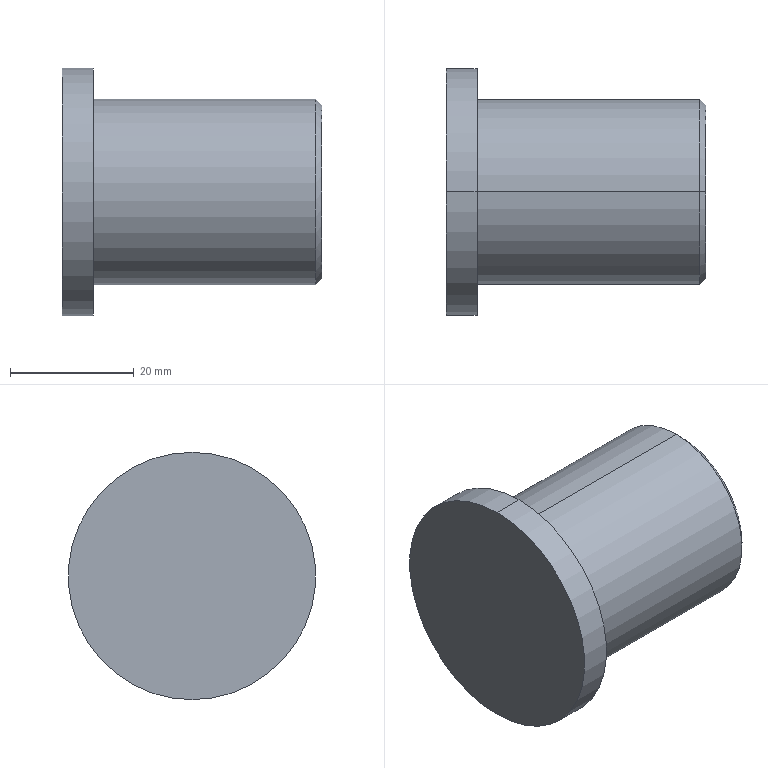Part | SolidWorks | features MBimport 1 | 1 solid | 18 faces | box 42 x 40 x 40 mm | volume 30182 mm3 | cylinder 8 | cone 6 | plane 4 | commonest cylinder face diameters 10.2 x2 12 x2 30 x2 40 x2
STEP:
#1=CARTESIAN_POINT('',(42.,17.24,-25.419));
#2=VERTEX_POINT('',#1);
#3=CARTESIAN_POINT('',(41.,17.24,-26.419));
#4=VERTEX_POINT('',#3);
#5=CARTESIAN_POINT('',(42.,17.24,-25.419));
#6=DIRECTION('',(-0.7071,0.,-0.7071));
#7=VECTOR('',#6,1000.);
#8=LINE('',#5,#7);
#9=EDGE_CURVE('',#2,#4,#8,.T.);
#10=ORIENTED_EDGE('',*,*,#9,.F.);
#11=CARTESIAN_POINT('',(42.,17.24,2.581));
#12=VERTEX_POINT('',#11);
#13=CARTESIAN_POINT('',(42.,17.24,-11.419));
#14=DIRECTION('',(1.,0.,0.));
#15=DIRECTION('',(0.,0.,-1.));
#16=AXIS2_PLACEMENT_3D('',#13,#14,#15);
#17=CIRCLE('',#16,14.);
#18=EDGE_CURVE('',#12,#2,#17,.T.);
#19=ORIENTED_EDGE('',*,*,#18,.F.);
#20=CARTESIAN_POINT('',(41.,17.24,3.581));
#21=VERTEX_POINT('',#20);
#22=CARTESIAN_POINT('',(42.,17.24,2.581));
#23=DIRECTION('',(-0.7071,0.,0.7071));
#24=VECTOR('',#23,1000.);
#25=LINE('',#22,#24);
#26=EDGE_CURVE('',#12,#21,#25,.T.);
#27=ORIENTED_EDGE('',*,*,#26,.T.);
#28=CARTESIAN_POINT('',(41.,17.24,-11.419));
#29=DIRECTION('',(-1.,0.,0.));
#30=DIRECTION('',(0.,0.,-1.));
#31=AXIS2_PLACEMENT_3D('',#28,#29,#30);
#32=CIRCLE('',#31,15.);
#33=EDGE_CURVE('',#4,#21,#32,.T.);
#34=ORIENTED_EDGE('',*,*,#33,.F.);
#35=EDGE_LOOP('',(#10,#19,#27,#34));
#36=FACE_OUTER_BOUND('',#35,.T.);
#37=CARTESIAN_POINT('',(42.,17.24,-11.419));
#38=DIRECTION('',(-1.,0.,0.));
#39=DIRECTION('',(0.,0.,1.));
#40=AXIS2_PLACEMENT_3D('',#37,#38,#39);
#41=CONICAL_SURFACE('',#40,14.,0.7854);
#42=ADVANCED_FACE('',(#36),#41,.T.);
#43=CARTESIAN_POINT('',(41.975,17.24,-5.419));
#44=VERTEX_POINT('',#43);
#45=CARTESIAN_POINT('',(42.,17.24,-5.394));
#46=VERTEX_POINT('',#45);
#47=CARTESIAN_POINT('',(42.,17.24,-5.394));
#48=DIRECTION('',(0.7071,0.,0.7071));
#49=VECTOR('',#48,1000.);
#50=LINE('',#47,#49);
#51=EDGE_CURVE('',#44,#46,#50,.T.);
#52=ORIENTED_EDGE('',*,*,#51,.F.);
#53=CARTESIAN_POINT('',(41.975,17.24,-17.419));
#54=VERTEX_POINT('',#53);
#55=CARTESIAN_POINT('',(41.975,17.24,-11.419));
#56=DIRECTION('',(1.,0.,0.));
#57=DIRECTION('',(0.,0.,-1.));
#58=AXIS2_PLACEMENT_3D('',#55,#56,#57);
#59=CIRCLE('',#58,6.);
#60=EDGE_CURVE('',#54,#44,#59,.T.);
#61=ORIENTED_EDGE('',*,*,#60,.F.);
#62=CARTESIAN_POINT('',(42.,17.24,-17.444));
#63=VERTEX_POINT('',#62);
#64=CARTESIAN_POINT('',(42.,17.24,-17.444));
#65=DIRECTION('',(0.7071,0.,-0.7071));
#66=VECTOR('',#65,1000.);
#67=LINE('',#64,#66);
#68=EDGE_CURVE('',#54,#63,#67,.T.);
#69=ORIENTED_EDGE('',*,*,#68,.T.);
#70=CARTESIAN_POINT('',(42.,17.24,-11.419));
#71=DIRECTION('',(1.,0.,0.));
#72=DIRECTION('',(0.,0.,-1.));
#73=AXIS2_PLACEMENT_3D('',#70,#71,#72);
#74=CIRCLE('',#73,6.025);
#75=EDGE_CURVE('',#63,#46,#74,.T.);
#76=ORIENTED_EDGE('',*,*,#75,.T.);
#77=EDGE_LOOP('',(#52,#61,#69,#76));
#78=FACE_OUTER_BOUND('',#77,.T.);
#79=CARTESIAN_POINT('',(42.,17.24,-11.419));
#80=DIRECTION('',(1.,0.,0.));
#81=DIRECTION('',(0.,0.,-1.));
#82=AXIS2_PLACEMENT_3D('',#79,#80,#81);
#83=CONICAL_SURFACE('',#82,6.025,0.7854);
#84=ADVANCED_FACE('',(#78),#83,.F.);
#85=CARTESIAN_POINT('',(27.,17.24,-5.419));
#86=VERTEX_POINT('',#85);
#87=CARTESIAN_POINT('',(42.,17.24,-5.419));
#88=DIRECTION('',(1.,0.,0.));
#89=VECTOR('',#88,1000.);
#90=LINE('',#87,#89);
#91=EDGE_CURVE('',#86,#44,#90,.T.);
#92=ORIENTED_EDGE('',*,*,#91,.F.);
#93=CARTESIAN_POINT('',(27.,17.24,-17.419));
#94=VERTEX_POINT('',#93);
#95=CARTESIAN_POINT('',(27.,17.24,-11.419));
#96=DIRECTION('',(1.,0.,0.));
#97=DIRECTION('',(0.,0.,-1.));
#98=AXIS2_PLACEMENT_3D('',#95,#96,#97);
#99=CIRCLE('',#98,6.);
#100=EDGE_CURVE('',#94,#86,#99,.T.);
#101=ORIENTED_EDGE('',*,*,#100,.F.);
#102=CARTESIAN_POINT('',(42.,17.24,-17.419));
#103=DIRECTION('',(1.,0.,0.));
#104=VECTOR('',#103,1000.);
#105=LINE('',#102,#104);
#106=EDGE_CURVE('',#94,#54,#105,.T.);
#107=ORIENTED_EDGE('',*,*,#106,.T.);
#108=ORIENTED_EDGE('',*,*,#60,.T.);
#109=EDGE_LOOP('',(#92,#101,#107,#108));
#110=FACE_OUTER_BOUND('',#109,.T.);
#111=CARTESIAN_POINT('',(42.,17.24,-11.419));
#112=DIRECTION('',(1.,0.,0.));
#113=DIRECTION('',(0.,0.,-1.));
#114=AXIS2_PLACEMENT_3D('',#111,#112,#113);
#115=CYLINDRICAL_SURFACE('',#114,6.);
#116=ADVANCED_FACE('',(#110),#115,.F.);
#117=CARTESIAN_POINT('',(27.,17.24,-16.519));
#118=VERTEX_POINT('',#117);
#119=CARTESIAN_POINT('',(27.,17.24,-6.319));
#120=VERTEX_POINT('',#119);
#121=CARTESIAN_POINT('',(27.,17.24,-11.419));
#122=DIRECTION('',(1.,0.,0.));
#123=DIRECTION('',(0.,0.,-1.));
#124=AXIS2_PLACEMENT_3D('',#121,#122,#123);
#125=CIRCLE('',#124,5.1);
#126=EDGE_CURVE('',#118,#120,#125,.T.);
#127=ORIENTED_EDGE('',*,*,#126,.F.);
#128=CARTESIAN_POINT('',(27.,17.24,-11.419));
#129=DIRECTION('',(1.,0.,0.));
#130=DIRECTION('',(0.,0.,-1.));
#131=AXIS2_PLACEMENT_3D('',#128,#129,#130);
#132=CIRCLE('',#131,5.1);
#133=EDGE_CURVE('',#120,#118,#132,.T.);
#134=ORIENTED_EDGE('',*,*,#133,.F.);
#135=EDGE_LOOP('',(#127,#134));
#136=FACE_BOUND('',#135,.T.);
#137=ORIENTED_EDGE('',*,*,#100,.T.);
#138=CARTESIAN_POINT('',(27.,17.24,-11.419));
#139=DIRECTION('',(1.,0.,0.));
#140=DIRECTION('',(0.,0.,-1.));
#141=AXIS2_PLACEMENT_3D('',#138,#139,#140);
#142=CIRCLE('',#141,6.);
#143=EDGE_CURVE('',#86,#94,#142,.T.);
#144=ORIENTED_EDGE('',*,*,#143,.T.);
#145=EDGE_LOOP('',(#137,#144));
#146=FACE_OUTER_BOUND('',#145,.T.);
#147=CARTESIAN_POINT('',(27.,22.34,-11.419));
#148=DIRECTION('',(-1.,0.,0.));
#149=DIRECTION('',(0.,0.,1.));
#150=AXIS2_PLACEMENT_3D('',#147,#148,#149);
#151=PLANE('',#150);
#152=ADVANCED_FACE('',(#136,#146),#151,.F.);
#153=CARTESIAN_POINT('',(21.75,17.24,-6.319));
#154=VERTEX_POINT('',#153);
#155=CARTESIAN_POINT('',(42.,17.24,-6.319));
#156=DIRECTION('',(1.,0.,0.));
#157=VECTOR('',#156,1000.);
#158=LINE('',#155,#157);
#159=EDGE_CURVE('',#154,#120,#158,.T.);
#160=ORIENTED_EDGE('',*,*,#159,.F.);
#161=CARTESIAN_POINT('',(21.75,17.24,-16.519));
#162=VERTEX_POINT('',#161);
#163=CARTESIAN_POINT('',(21.75,17.24,-11.419));
#164=DIRECTION('',(1.,0.,0.));
#165=DIRECTION('',(0.,0.,-1.));
#166=AXIS2_PLACEMENT_3D('',#163,#164,#165);
#167=CIRCLE('',#166,5.1);
#168=EDGE_CURVE('',#162,#154,#167,.T.);
#169=ORIENTED_EDGE('',*,*,#168,.F.);
#170=CARTESIAN_POINT('',(42.,17.24,-16.519));
#171=DIRECTION('',(1.,0.,0.));
#172=VECTOR('',#171,1000.);
#173=LINE('',#170,#172);
#174=EDGE_CURVE('',#162,#118,#173,.T.);
#175=ORIENTED_EDGE('',*,*,#174,.T.);
#176=ORIENTED_EDGE('',*,*,#126,.T.);
#177=EDGE_LOOP('',(#160,#169,#175,#176));
#178=FACE_OUTER_BOUND('',#177,.T.);
#179=CARTESIAN_POINT('',(42.,17.24,-11.419));
#180=DIRECTION('',(1.,0.,0.));
#181=DIRECTION('',(0.,0.,-1.));
#182=AXIS2_PLACEMENT_3D('',#179,#180,#181);
#183=CYLINDRICAL_SURFACE('',#182,5.1);
#184=ADVANCED_FACE('',(#178),#183,.F.);
#185=CARTESIAN_POINT('',(18.686,17.24,-11.419));
#186=VERTEX_POINT('',#185);
#187=CARTESIAN_POINT('',(21.75,17.24,-6.319));
#188=DIRECTION('',(0.515,0.,0.8572));
#189=VECTOR('',#188,1000.);
#190=LINE('',#187,#189);
#191=EDGE_CURVE('',#186,#154,#190,.T.);
#192=ORIENTED_EDGE('',*,*,#191,.F.);
#193=CARTESIAN_POINT('',(21.75,17.24,-16.519));
#194=DIRECTION('',(0.515,0.,-0.8572));
#195=VECTOR('',#194,1000.);
#196=LINE('',#193,#195);
#197=EDGE_CURVE('',#186,#162,#196,.T.);
#198=ORIENTED_EDGE('',*,*,#197,.T.);
#199=ORIENTED_EDGE('',*,*,#168,.T.);
#200=EDGE_LOOP('',(#192,#198,#199));
#201=FACE_OUTER_BOUND('',#200,.T.);
#202=CARTESIAN_POINT('',(21.75,17.24,-11.419));
#203=DIRECTION('',(1.,0.,0.));
#204=DIRECTION('',(0.,0.,-1.));
#205=AXIS2_PLACEMENT_3D('',#202,#203,#204);
#206=CONICAL_SURFACE('',#205,5.1,1.03);
#207=ADVANCED_FACE('',(#201),#206,.F.);
#208=ORIENTED_EDGE('',*,*,#75,.F.);
#209=CARTESIAN_POINT('',(42.,17.24,-11.419));
#210=DIRECTION('',(1.,0.,0.));
#211=DIRECTION('',(0.,0.,-1.));
#212=AXIS2_PLACEMENT_3D('',#209,#210,#211);
#213=CIRCLE('',#212,6.025);
#214=EDGE_CURVE('',#46,#63,#213,.T.);
#215=ORIENTED_EDGE('',*,*,#214,.F.);
#216=EDGE_LOOP('',(#208,#215));
#217=FACE_BOUND('',#216,.T.);
#218=ORIENTED_EDGE('',*,*,#18,.T.);
#219=CARTESIAN_POINT('',(42.,17.24,-11.419));
#220=DIRECTION('',(1.,0.,0.));
#221=DIRECTION('',(0.,0.,-1.));
#222=AXIS2_PLACEMENT_3D('',#219,#220,#221);
#223=CIRCLE('',#222,14.);
#224=EDGE_CURVE('',#2,#12,#223,.T.);
#225=ORIENTED_EDGE('',*,*,#224,.T.);
#226=EDGE_LOOP('',(#218,#225));
#227=FACE_OUTER_BOUND('',#226,.T.);
#228=CARTESIAN_POINT('',(42.,17.24,-11.419));
#229=DIRECTION('',(1.,0.,0.));
#230=DIRECTION('',(0.,1.,0.));
#231=AXIS2_PLACEMENT_3D('',#228,#229,#230);
#232=PLANE('',#231);
#233=ADVANCED_FACE('',(#217,#227),#232,.T.);
#234=CARTESIAN_POINT('',(5.,17.24,-26.419));
#235=VERTEX_POINT('',#234);
#236=CARTESIAN_POINT('',(42.,17.24,-26.419));
#237=DIRECTION('',(-1.,0.,0.));
#238=VECTOR('',#237,1000.);
#239=LINE('',#236,#238);
#240=EDGE_CURVE('',#4,#235,#239,.T.);
#241=ORIENTED_EDGE('',*,*,#240,.F.);
#242=ORIENTED_EDGE('',*,*,#33,.T.);
#243=CARTESIAN_POINT('',(5.,17.24,3.581));
#244=VERTEX_POINT('',#243);
#245=CARTESIAN_POINT('',(42.,17.24,3.581));
#246=DIRECTION('',(-1.,0.,0.));
#247=VECTOR('',#246,1000.);
#248=LINE('',#245,#247);
#249=EDGE_CURVE('',#21,#244,#248,.T.);
#250=ORIENTED_EDGE('',*,*,#249,.T.);
#251=CARTESIAN_POINT('',(5.,17.24,-11.419));
#252=DIRECTION('',(1.,0.,0.));
#253=DIRECTION('',(0.,0.,-1.));
#254=AXIS2_PLACEMENT_3D('',#251,#252,#253);
#255=CIRCLE('',#254,15.);
#256=EDGE_CURVE('',#244,#235,#255,.T.);
#257=ORIENTED_EDGE('',*,*,#256,.T.);
#258=EDGE_LOOP('',(#241,#242,#250,#257));
#259=FACE_OUTER_BOUND('',#258,.T.);
#260=CARTESIAN_POINT('',(42.,17.24,-11.419));
#261=DIRECTION('',(-1.,0.,0.));
#262=DIRECTION('',(0.,0.,1.));
#263=AXIS2_PLACEMENT_3D('',#260,#261,#262);
#264=CYLINDRICAL_SURFACE('',#263,15.);
#265=ADVANCED_FACE('',(#259),#264,.T.);
#266=CARTESIAN_POINT('',(0.,17.24,8.581));
#267=VERTEX_POINT('',#266);
#268=CARTESIAN_POINT('',(0.,17.24,-31.419));
#269=VERTEX_POINT('',#268);
#270=CARTESIAN_POINT('',(0.,17.24,-11.419));
#271=DIRECTION('',(1.,0.,0.));
#272=DIRECTION('',(0.,0.,-1.));
#273=AXIS2_PLACEMENT_3D('',#270,#271,#272);
#274=CIRCLE('',#273,20.);
#275=EDGE_CURVE('',#267,#269,#274,.T.);
#276=ORIENTED_EDGE('',*,*,#275,.F.);
#277=CARTESIAN_POINT('',(0.,17.24,-11.419));
#278=DIRECTION('',(1.,0.,0.));
#279=DIRECTION('',(0.,0.,-1.));
#280=AXIS2_PLACEMENT_3D('',#277,#278,#279);
#281=CIRCLE('',#280,20.);
#282=EDGE_CURVE('',#269,#267,#281,.T.);
#283=ORIENTED_EDGE('',*,*,#282,.F.);
#284=EDGE_LOOP('',(#276,#283));
#285=FACE_OUTER_BOUND('',#284,.T.);
#286=CARTESIAN_POINT('',(0.,17.24,-11.419));
#287=DIRECTION('',(1.,0.,0.));
#288=DIRECTION('',(0.,1.,0.));
#289=AXIS2_PLACEMENT_3D('',#286,#287,#288);
#290=PLANE('',#289);
#291=ADVANCED_FACE('',(#285),#290,.F.);
#292=ORIENTED_EDGE('',*,*,#256,.F.);
#293=CARTESIAN_POINT('',(5.,17.24,-11.419));
#294=DIRECTION('',(1.,0.,0.));
#295=DIRECTION('',(0.,0.,-1.));
#296=AXIS2_PLACEMENT_3D('',#293,#294,#295);
#297=CIRCLE('',#296,15.);
#298=EDGE_CURVE('',#235,#244,#297,.T.);
#299=ORIENTED_EDGE('',*,*,#298,.F.);
#300=EDGE_LOOP('',(#292,#299));
#301=FACE_BOUND('',#300,.T.);
#302=CARTESIAN_POINT('',(5.,17.24,8.581));
#303=VERTEX_POINT('',#302);
#304=CARTESIAN_POINT('',(5.,17.24,-31.419));
#305=VERTEX_POINT('',#304);
#306=CARTESIAN_POINT('',(5.,17.24,-11.419));
#307=DIRECTION('',(1.,0.,0.));
#308=DIRECTION('',(0.,0.,-1.));
#309=AXIS2_PLACEMENT_3D('',#306,#307,#308);
#310=CIRCLE('',#309,20.);
#311=EDGE_CURVE('',#303,#305,#310,.T.);
#312=ORIENTED_EDGE('',*,*,#311,.T.);
#313=CARTESIAN_POINT('',(5.,17.24,-11.419));
#314=DIRECTION('',(1.,0.,0.));
#315=DIRECTION('',(0.,0.,-1.));
#316=AXIS2_PLACEMENT_3D('',#313,#314,#315);
#317=CIRCLE('',#316,20.);
#318=EDGE_CURVE('',#305,#303,#317,.T.);
#319=ORIENTED_EDGE('',*,*,#318,.T.);
#320=EDGE_LOOP('',(#312,#319));
#321=FACE_OUTER_BOUND('',#320,.T.);
#322=CARTESIAN_POINT('',(5.,17.24,-11.419));
#323=DIRECTION('',(1.,0.,0.));
#324=DIRECTION('',(0.,1.,0.));
#325=AXIS2_PLACEMENT_3D('',#322,#323,#324);
#326=PLANE('',#325);
#327=ADVANCED_FACE('',(#301,#321),#326,.T.);
#328=CARTESIAN_POINT('',(5.,17.24,-31.419));
#329=DIRECTION('',(-1.,0.,0.));
#330=VECTOR('',#329,1000.);
#331=LINE('',#328,#330);
#332=EDGE_CURVE('',#305,#269,#331,.T.);
#333=ORIENTED_EDGE('',*,*,#332,.F.);
#334=ORIENTED_EDGE('',*,*,#311,.F.);
#335=CARTESIAN_POINT('',(5.,17.24,8.581));
#336=DIRECTION('',(-1.,0.,0.));
#337=VECTOR('',#336,1000.);
#338=LINE('',#335,#337);
#339=EDGE_CURVE('',#303,#267,#338,.T.);
#340=ORIENTED_EDGE('',*,*,#339,.T.);
#341=ORIENTED_EDGE('',*,*,#275,.T.);
#342=EDGE_LOOP('',(#333,#334,#340,#341));
#343=FACE_OUTER_BOUND('',#342,.T.);
#344=CARTESIAN_POINT('',(5.,17.24,-11.419));
#345=DIRECTION('',(-1.,0.,0.));
#346=DIRECTION('',(0.,0.,1.));
#347=AXIS2_PLACEMENT_3D('',#344,#345,#346);
#348=CYLINDRICAL_SURFACE('',#347,20.);
#349=ADVANCED_FACE('',(#343),#348,.T.);
#350=ORIENTED_EDGE('',*,*,#318,.F.);
#351=ORIENTED_EDGE('',*,*,#332,.T.);
#352=ORIENTED_EDGE('',*,*,#282,.T.);
#353=ORIENTED_EDGE('',*,*,#339,.F.);
#354=EDGE_LOOP('',(#350,#351,#352,#353));
#355=FACE_OUTER_BOUND('',#354,.T.);
#356=CARTESIAN_POINT('',(5.,17.24,-11.419));
#357=DIRECTION('',(-1.,0.,0.));
#358=DIRECTION('',(0.,0.,1.));
#359=AXIS2_PLACEMENT_3D('',#356,#357,#358);
#360=CYLINDRICAL_SURFACE('',#359,20.);
#361=ADVANCED_FACE('',(#355),#360,.T.);
#362=CARTESIAN_POINT('',(41.,17.24,-11.419));
#363=DIRECTION('',(-1.,0.,0.));
#364=DIRECTION('',(0.,0.,-1.));
#365=AXIS2_PLACEMENT_3D('',#362,#363,#364);
#366=CIRCLE('',#365,15.);
#367=EDGE_CURVE('',#21,#4,#366,.T.);
#368=ORIENTED_EDGE('',*,*,#367,.T.);
#369=ORIENTED_EDGE('',*,*,#240,.T.);
#370=ORIENTED_EDGE('',*,*,#298,.T.);
#371=ORIENTED_EDGE('',*,*,#249,.F.);
#372=EDGE_LOOP('',(#368,#369,#370,#371));
#373=FACE_OUTER_BOUND('',#372,.T.);
#374=CARTESIAN_POINT('',(42.,17.24,-11.419));
#375=DIRECTION('',(-1.,0.,0.));
#376=DIRECTION('',(0.,0.,1.));
#377=AXIS2_PLACEMENT_3D('',#374,#375,#376);
#378=CYLINDRICAL_SURFACE('',#377,15.);
#379=ADVANCED_FACE('',(#373),#378,.T.);
#380=ORIENTED_EDGE('',*,*,#197,.F.);
#381=ORIENTED_EDGE('',*,*,#191,.T.);
#382=CARTESIAN_POINT('',(21.75,17.24,-11.419));
#383=DIRECTION('',(1.,0.,0.));
#384=DIRECTION('',(0.,0.,-1.));
#385=AXIS2_PLACEMENT_3D('',#382,#383,#384);
#386=CIRCLE('',#385,5.1);
#387=EDGE_CURVE('',#154,#162,#386,.T.);
#388=ORIENTED_EDGE('',*,*,#387,.T.);
#389=EDGE_LOOP('',(#380,#381,#388));
#390=FACE_OUTER_BOUND('',#389,.T.);
#391=CARTESIAN_POINT('',(21.75,17.24,-11.419));
#392=DIRECTION('',(1.,0.,0.));
#393=DIRECTION('',(0.,0.,-1.));
#394=AXIS2_PLACEMENT_3D('',#391,#392,#393);
#395=CONICAL_SURFACE('',#394,5.1,1.03);
#396=ADVANCED_FACE('',(#390),#395,.F.);
#397=ORIENTED_EDGE('',*,*,#387,.F.);
#398=ORIENTED_EDGE('',*,*,#159,.T.);
#399=ORIENTED_EDGE('',*,*,#133,.T.);
#400=ORIENTED_EDGE('',*,*,#174,.F.);
#401=EDGE_LOOP('',(#397,#398,#399,#400));
#402=FACE_OUTER_BOUND('',#401,.T.);
#403=CARTESIAN_POINT('',(42.,17.24,-11.419));
#404=DIRECTION('',(1.,0.,0.));
#405=DIRECTION('',(0.,0.,-1.));
#406=AXIS2_PLACEMENT_3D('',#403,#404,#405);
#407=CYLINDRICAL_SURFACE('',#406,5.1);
#408=ADVANCED_FACE('',(#402),#407,.F.);
#409=ORIENTED_EDGE('',*,*,#143,.F.);
#410=ORIENTED_EDGE('',*,*,#91,.T.);
#411=CARTESIAN_POINT('',(41.975,17.24,-11.419));
#412=DIRECTION('',(1.,0.,0.));
#413=DIRECTION('',(0.,0.,-1.));
#414=AXIS2_PLACEMENT_3D('',#411,#412,#413);
#415=CIRCLE('',#414,6.);
#416=EDGE_CURVE('',#44,#54,#415,.T.);
#417=ORIENTED_EDGE('',*,*,#416,.T.);
#418=ORIENTED_EDGE('',*,*,#106,.F.);
#419=EDGE_LOOP('',(#409,#410,#417,#418));
#420=FACE_OUTER_BOUND('',#419,.T.);
#421=CARTESIAN_POINT('',(42.,17.24,-11.419));
#422=DIRECTION('',(1.,0.,0.));
#423=DIRECTION('',(0.,0.,-1.));
#424=AXIS2_PLACEMENT_3D('',#421,#422,#423);
#425=CYLINDRICAL_SURFACE('',#424,6.);
#426=ADVANCED_FACE('',(#420),#425,.F.);
#427=ORIENTED_EDGE('',*,*,#416,.F.);
#428=ORIENTED_EDGE('',*,*,#51,.T.);
#429=ORIENTED_EDGE('',*,*,#214,.T.);
#430=ORIENTED_EDGE('',*,*,#68,.F.);
#431=EDGE_LOOP('',(#427,#428,#429,#430));
#432=FACE_OUTER_BOUND('',#431,.T.);
#433=CARTESIAN_POINT('',(42.,17.24,-11.419));
#434=DIRECTION('',(1.,0.,0.));
#435=DIRECTION('',(0.,0.,-1.));
#436=AXIS2_PLACEMENT_3D('',#433,#434,#435);
#437=CONICAL_SURFACE('',#436,6.025,0.7854);
#438=ADVANCED_FACE('',(#432),#437,.F.);
#439=ORIENTED_EDGE('',*,*,#224,.F.);
#440=ORIENTED_EDGE('',*,*,#9,.T.);
#441=ORIENTED_EDGE('',*,*,#367,.F.);
#442=ORIENTED_EDGE('',*,*,#26,.F.);
#443=EDGE_LOOP('',(#439,#440,#441,#442));
#444=FACE_OUTER_BOUND('',#443,.T.);
#445=CARTESIAN_POINT('',(42.,17.24,-11.419));
#446=DIRECTION('',(-1.,0.,0.));
#447=DIRECTION('',(0.,0.,1.));
#448=AXIS2_PLACEMENT_3D('',#445,#446,#447);
#449=CONICAL_SURFACE('',#448,14.,0.7854);
#450=ADVANCED_FACE('',(#444),#449,.T.);
#451=CLOSED_SHELL('',(#42,#84,#116,#152,#184,#207,#233,#265,#291,#327,#349,#361,#379,#396,#408,#426,#438,#450));
#452=MANIFOLD_SOLID_BREP('',#451);
#453=CARTESIAN_POINT('',(0.,0.,0.));
#454=DIRECTION('',(0.,0.,1.));
#455=DIRECTION('',(1.,0.,0.));
#456=AXIS2_PLACEMENT_3D('',#453,#454,#455);
#457=(LENGTH_UNIT()NAMED_UNIT(*)SI_UNIT(.MILLI.,.METRE.));
#458=UNCERTAINTY_MEASURE_WITH_UNIT(LENGTH_MEASURE(0.00001),#457,'','');
#459=(NAMED_UNIT(*)PLANE_ANGLE_UNIT()SI_UNIT($,.RADIAN.));
#460=(NAMED_UNIT(*)SI_UNIT($,.STERADIAN.)SOLID_ANGLE_UNIT());
#461=(GEOMETRIC_REPRESENTATION_CONTEXT(3)GLOBAL_UNCERTAINTY_ASSIGNED_CONTEXT((#458))GLOBAL_UNIT_ASSIGNED_CONTEXT((#457,#459,#460))REPRESENTATION_CONTEXT('',''));
#462=ADVANCED_BREP_SHAPE_REPRESENTATION('',(#452,#456),#461);